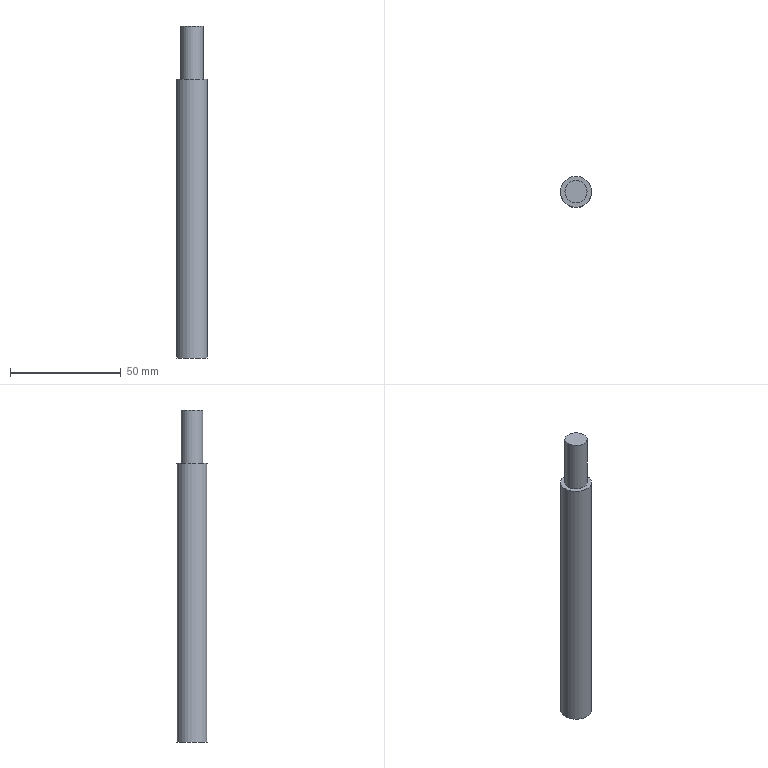Part | NX | features solid 2 | 1 solid | 5 faces | box 14 x 14 x 150 mm | volume 21281 mm3 | plane 3 | cylinder 2 | commonest cylinder face diameters 10 x1 14 x1
STEP:
#1=CARTESIAN_POINT('',(8.,255.,-145.));
#2=VERTEX_POINT('',#1);
#3=CARTESIAN_POINT('',(15.,255.,-145.));
#4=DIRECTION('',(0.,0.,-1.));
#5=DIRECTION('',(-1.,0.,0.));
#6=AXIS2_PLACEMENT_3D('',#3,#4,#5);
#7=CIRCLE('',#6,7.);
#8=EDGE_CURVE('',#2,#2,#7,.F.);
#9=ORIENTED_EDGE('',*,*,#8,.F.);
#10=EDGE_LOOP('',(#9));
#11=FACE_BOUND('',#10,.T.);
#12=CARTESIAN_POINT('',(15.,255.,-145.));
#13=DIRECTION('',(0.,0.,-1.));
#14=DIRECTION('',(-1.,0.,0.));
#15=AXIS2_PLACEMENT_3D('',#12,#13,#14);
#16=PLANE('',#15);
#17=ADVANCED_FACE('',(#11),#16,.T.);
#18=CARTESIAN_POINT('',(8.,255.,-19.));
#19=VERTEX_POINT('',#18);
#20=CARTESIAN_POINT('',(15.,255.,-19.));
#21=DIRECTION('',(0.,0.,-1.));
#22=DIRECTION('',(-1.,0.,0.));
#23=AXIS2_PLACEMENT_3D('',#20,#21,#22);
#24=CIRCLE('',#23,7.);
#25=EDGE_CURVE('',#19,#19,#24,.F.);
#26=ORIENTED_EDGE('',*,*,#25,.F.);
#27=EDGE_LOOP('',(#26));
#28=FACE_BOUND('',#27,.T.);
#29=ORIENTED_EDGE('',*,*,#8,.T.);
#30=EDGE_LOOP('',(#29));
#31=FACE_BOUND('',#30,.T.);
#32=CARTESIAN_POINT('',(15.,255.,5.));
#33=DIRECTION('',(0.,0.,-1.));
#34=DIRECTION('',(-1.,0.,0.));
#35=AXIS2_PLACEMENT_3D('',#32,#33,#34);
#36=CYLINDRICAL_SURFACE('',#35,7.);
#37=ADVANCED_FACE('',(#28,#31),#36,.T.);
#38=CARTESIAN_POINT('',(10.,255.,-19.));
#39=VERTEX_POINT('',#38);
#40=CARTESIAN_POINT('',(15.,255.,-19.));
#41=DIRECTION('',(0.,0.,-1.));
#42=DIRECTION('',(-1.,0.,0.));
#43=AXIS2_PLACEMENT_3D('',#40,#41,#42);
#44=CIRCLE('',#43,5.);
#45=EDGE_CURVE('',#39,#39,#44,.F.);
#46=ORIENTED_EDGE('',*,*,#45,.F.);
#47=EDGE_LOOP('',(#46));
#48=FACE_BOUND('',#47,.T.);
#49=ORIENTED_EDGE('',*,*,#25,.T.);
#50=EDGE_LOOP('',(#49));
#51=FACE_BOUND('',#50,.T.);
#52=CARTESIAN_POINT('',(15.,207.5,-19.));
#53=DIRECTION('',(0.,0.,-1.));
#54=DIRECTION('',(-1.,0.,0.));
#55=AXIS2_PLACEMENT_3D('',#52,#53,#54);
#56=PLANE('',#55);
#57=ADVANCED_FACE('',(#48,#51),#56,.F.);
#58=CARTESIAN_POINT('',(20.,255.,5.));
#59=VERTEX_POINT('',#58);
#60=CARTESIAN_POINT('',(15.,255.,5.));
#61=DIRECTION('',(0.,0.,1.));
#62=DIRECTION('',(1.,0.,0.));
#63=AXIS2_PLACEMENT_3D('',#60,#61,#62);
#64=CIRCLE('',#63,5.);
#65=EDGE_CURVE('',#59,#59,#64,.F.);
#66=ORIENTED_EDGE('',*,*,#65,.F.);
#67=EDGE_LOOP('',(#66));
#68=FACE_BOUND('',#67,.T.);
#69=CARTESIAN_POINT('',(15.,195.,5.));
#70=DIRECTION('',(0.,0.,1.));
#71=DIRECTION('',(1.,0.,0.));
#72=AXIS2_PLACEMENT_3D('',#69,#70,#71);
#73=PLANE('',#72);
#74=ADVANCED_FACE('',(#68),#73,.T.);
#75=ORIENTED_EDGE('',*,*,#65,.T.);
#76=EDGE_LOOP('',(#75));
#77=FACE_BOUND('',#76,.T.);
#78=ORIENTED_EDGE('',*,*,#45,.T.);
#79=EDGE_LOOP('',(#78));
#80=FACE_BOUND('',#79,.T.);
#81=CARTESIAN_POINT('',(15.,255.,5.));
#82=DIRECTION('',(0.,0.,-1.));
#83=DIRECTION('',(-1.,0.,0.));
#84=AXIS2_PLACEMENT_3D('',#81,#82,#83);
#85=CYLINDRICAL_SURFACE('',#84,5.);
#86=ADVANCED_FACE('',(#77,#80),#85,.T.);
#87=CLOSED_SHELL('',(#17,#37,#57,#74,#86));
#88=MANIFOLD_SOLID_BREP('',#87);
#89=(LENGTH_UNIT()NAMED_UNIT(*)SI_UNIT(.MILLI.,.METRE.));
#90=UNCERTAINTY_MEASURE_WITH_UNIT(LENGTH_MEASURE(0.00001),#89,'','');
#91=(NAMED_UNIT(*)PLANE_ANGLE_UNIT()SI_UNIT($,.RADIAN.));
#92=(NAMED_UNIT(*)SI_UNIT($,.STERADIAN.)SOLID_ANGLE_UNIT());
#93=(GEOMETRIC_REPRESENTATION_CONTEXT(3)GLOBAL_UNCERTAINTY_ASSIGNED_CONTEXT((#90))GLOBAL_UNIT_ASSIGNED_CONTEXT((#89,#91,#92))REPRESENTATION_CONTEXT('',''));
#94=ADVANCED_BREP_SHAPE_REPRESENTATION('',(#88),#93);